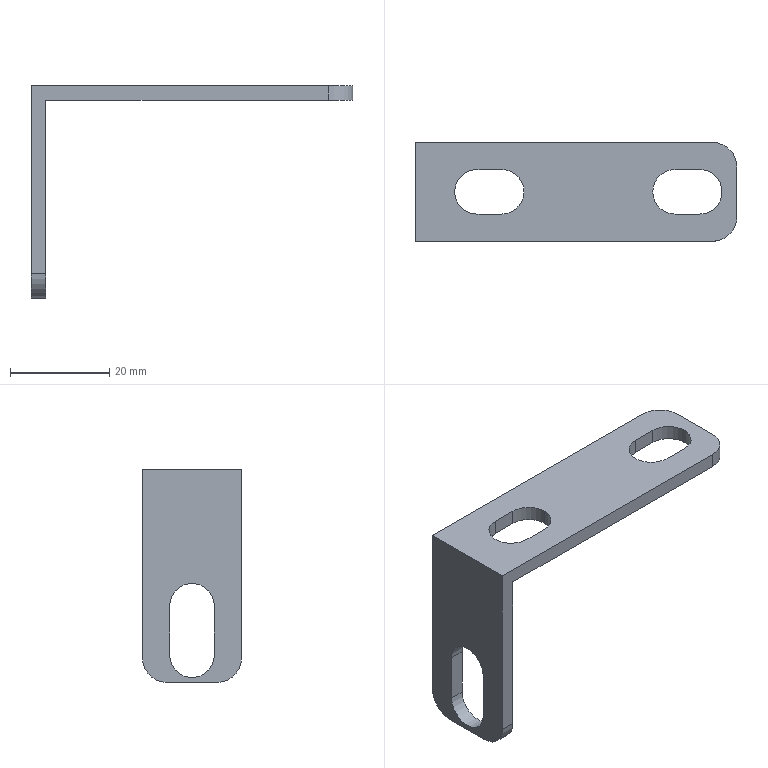Part | SolidWorks | features BaseBody 1 | 1 solid | 26 faces | box 65 x 20 x 43 mm | volume 5123 mm3 | plane 14 | cylinder 12 | commonest cylinder face diameters 9 x8 10 x4
STEP:
#1=CARTESIAN_POINT('',(15.5,0.,3.));
#2=VERTEX_POINT('',#1);
#3=CARTESIAN_POINT('',(20.,4.5,3.));
#4=VERTEX_POINT('',#3);
#5=CARTESIAN_POINT('',(20.,0.,3.));
#6=DIRECTION('',(0.,0.,-1.));
#7=DIRECTION('',(-1.,0.,0.));
#8=AXIS2_PLACEMENT_3D('',#5,#6,#7);
#9=CIRCLE('',#8,4.5);
#10=EDGE_CURVE('',#2,#4,#9,.T.);
#11=ORIENTED_EDGE('',*,*,#10,.F.);
#12=CARTESIAN_POINT('',(15.5,0.,0.));
#13=VERTEX_POINT('',#12);
#14=CARTESIAN_POINT('',(15.5,0.,3.));
#15=DIRECTION('',(0.,0.,-1.));
#16=VECTOR('',#15,1000.);
#17=LINE('',#14,#16);
#18=EDGE_CURVE('',#2,#13,#17,.T.);
#19=ORIENTED_EDGE('',*,*,#18,.T.);
#20=CARTESIAN_POINT('',(20.,4.5,0.));
#21=VERTEX_POINT('',#20);
#22=CARTESIAN_POINT('',(20.,0.,0.));
#23=DIRECTION('',(0.,0.,1.));
#24=DIRECTION('',(-1.,0.,0.));
#25=AXIS2_PLACEMENT_3D('',#22,#23,#24);
#26=CIRCLE('',#25,4.5);
#27=EDGE_CURVE('',#21,#13,#26,.T.);
#28=ORIENTED_EDGE('',*,*,#27,.F.);
#29=CARTESIAN_POINT('',(20.,4.5,3.));
#30=DIRECTION('',(0.,0.,1.));
#31=VECTOR('',#30,1000.);
#32=LINE('',#29,#31);
#33=EDGE_CURVE('',#21,#4,#32,.T.);
#34=ORIENTED_EDGE('',*,*,#33,.T.);
#35=EDGE_LOOP('',(#11,#19,#28,#34));
#36=FACE_OUTER_BOUND('',#35,.T.);
#37=CARTESIAN_POINT('',(20.,0.,3.));
#38=DIRECTION('',(0.,0.,-1.));
#39=DIRECTION('',(-1.,0.,0.));
#40=AXIS2_PLACEMENT_3D('',#37,#38,#39);
#41=CYLINDRICAL_SURFACE('',#40,4.5);
#42=ADVANCED_FACE('',(#36),#41,.F.);
#43=CARTESIAN_POINT('',(-10.5,0.,0.));
#44=VERTEX_POINT('',#43);
#45=CARTESIAN_POINT('',(-15.,4.5,0.));
#46=VERTEX_POINT('',#45);
#47=CARTESIAN_POINT('',(-15.,0.,0.));
#48=DIRECTION('',(0.,0.,1.));
#49=DIRECTION('',(1.,0.,0.));
#50=AXIS2_PLACEMENT_3D('',#47,#48,#49);
#51=CIRCLE('',#50,4.5);
#52=EDGE_CURVE('',#44,#46,#51,.T.);
#53=ORIENTED_EDGE('',*,*,#52,.F.);
#54=CARTESIAN_POINT('',(-10.5,0.,3.));
#55=VERTEX_POINT('',#54);
#56=CARTESIAN_POINT('',(-10.5,0.,-40.));
#57=DIRECTION('',(0.,0.,1.));
#58=VECTOR('',#57,1000.);
#59=LINE('',#56,#58);
#60=EDGE_CURVE('',#44,#55,#59,.T.);
#61=ORIENTED_EDGE('',*,*,#60,.T.);
#62=CARTESIAN_POINT('',(-15.,4.5,3.));
#63=VERTEX_POINT('',#62);
#64=CARTESIAN_POINT('',(-15.,0.,3.));
#65=DIRECTION('',(0.,0.,-1.));
#66=DIRECTION('',(1.,0.,0.));
#67=AXIS2_PLACEMENT_3D('',#64,#65,#66);
#68=CIRCLE('',#67,4.5);
#69=EDGE_CURVE('',#63,#55,#68,.T.);
#70=ORIENTED_EDGE('',*,*,#69,.F.);
#71=CARTESIAN_POINT('',(-15.,4.5,-40.));
#72=DIRECTION('',(0.,0.,1.));
#73=VECTOR('',#72,1000.);
#74=LINE('',#71,#73);
#75=EDGE_CURVE('',#46,#63,#74,.T.);
#76=ORIENTED_EDGE('',*,*,#75,.F.);
#77=EDGE_LOOP('',(#53,#61,#70,#76));
#78=FACE_OUTER_BOUND('',#77,.T.);
#79=CARTESIAN_POINT('',(-15.,0.,-40.));
#80=DIRECTION('',(0.,0.,1.));
#81=DIRECTION('',(1.,0.,0.));
#82=AXIS2_PLACEMENT_3D('',#79,#80,#81);
#83=CYLINDRICAL_SURFACE('',#82,4.5);
#84=ADVANCED_FACE('',(#78),#83,.F.);
#85=CARTESIAN_POINT('',(20.,-4.5,3.));
#86=VERTEX_POINT('',#85);
#87=CARTESIAN_POINT('',(20.,0.,3.));
#88=DIRECTION('',(0.,0.,-1.));
#89=DIRECTION('',(-1.,0.,0.));
#90=AXIS2_PLACEMENT_3D('',#87,#88,#89);
#91=CIRCLE('',#90,4.5);
#92=EDGE_CURVE('',#86,#2,#91,.T.);
#93=ORIENTED_EDGE('',*,*,#92,.T.);
#94=ORIENTED_EDGE('',*,*,#10,.T.);
#95=CARTESIAN_POINT('',(25.,4.5,3.));
#96=VERTEX_POINT('',#95);
#97=CARTESIAN_POINT('',(0.,4.5,3.));
#98=DIRECTION('',(1.,0.,0.));
#99=VECTOR('',#98,1000.);
#100=LINE('',#97,#99);
#101=EDGE_CURVE('',#4,#96,#100,.T.);
#102=ORIENTED_EDGE('',*,*,#101,.T.);
#103=CARTESIAN_POINT('',(25.,-4.5,3.));
#104=VERTEX_POINT('',#103);
#105=CARTESIAN_POINT('',(25.,0.,3.));
#106=DIRECTION('',(0.,0.,-1.));
#107=DIRECTION('',(-1.,0.,0.));
#108=AXIS2_PLACEMENT_3D('',#105,#106,#107);
#109=CIRCLE('',#108,4.5);
#110=EDGE_CURVE('',#96,#104,#109,.T.);
#111=ORIENTED_EDGE('',*,*,#110,.T.);
#112=CARTESIAN_POINT('',(0.,-4.5,3.));
#113=DIRECTION('',(-1.,0.,0.));
#114=VECTOR('',#113,1000.);
#115=LINE('',#112,#114);
#116=EDGE_CURVE('',#104,#86,#115,.T.);
#117=ORIENTED_EDGE('',*,*,#116,.T.);
#118=EDGE_LOOP('',(#93,#94,#102,#111,#117));
#119=FACE_BOUND('',#118,.T.);
#120=CARTESIAN_POINT('',(27.5,10.,3.));
#121=VERTEX_POINT('',#120);
#122=CARTESIAN_POINT('',(-32.5,10.,3.));
#123=VERTEX_POINT('',#122);
#124=CARTESIAN_POINT('',(0.,10.,3.));
#125=DIRECTION('',(-1.,0.,0.));
#126=VECTOR('',#125,1000.);
#127=LINE('',#124,#126);
#128=EDGE_CURVE('',#121,#123,#127,.T.);
#129=ORIENTED_EDGE('',*,*,#128,.T.);
#130=CARTESIAN_POINT('',(-32.5,-10.,3.));
#131=VERTEX_POINT('',#130);
#132=CARTESIAN_POINT('',(-32.5,0.,3.));
#133=DIRECTION('',(0.,-1.,0.));
#134=VECTOR('',#133,1000.);
#135=LINE('',#132,#134);
#136=EDGE_CURVE('',#123,#131,#135,.T.);
#137=ORIENTED_EDGE('',*,*,#136,.T.);
#138=CARTESIAN_POINT('',(27.5,-10.,3.));
#139=VERTEX_POINT('',#138);
#140=CARTESIAN_POINT('',(0.,-10.,3.));
#141=DIRECTION('',(1.,0.,0.));
#142=VECTOR('',#141,1000.);
#143=LINE('',#140,#142);
#144=EDGE_CURVE('',#131,#139,#143,.T.);
#145=ORIENTED_EDGE('',*,*,#144,.T.);
#146=CARTESIAN_POINT('',(32.5,-5.,3.));
#147=VERTEX_POINT('',#146);
#148=CARTESIAN_POINT('',(27.5,-5.,3.));
#149=DIRECTION('',(0.,0.,1.));
#150=DIRECTION('',(-1.,0.,0.));
#151=AXIS2_PLACEMENT_3D('',#148,#149,#150);
#152=CIRCLE('',#151,5.);
#153=EDGE_CURVE('',#139,#147,#152,.T.);
#154=ORIENTED_EDGE('',*,*,#153,.T.);
#155=CARTESIAN_POINT('',(32.5,5.,3.));
#156=VERTEX_POINT('',#155);
#157=CARTESIAN_POINT('',(32.5,0.,3.));
#158=DIRECTION('',(0.,1.,0.));
#159=VECTOR('',#158,1000.);
#160=LINE('',#157,#159);
#161=EDGE_CURVE('',#147,#156,#160,.T.);
#162=ORIENTED_EDGE('',*,*,#161,.T.);
#163=CARTESIAN_POINT('',(27.5,5.,3.));
#164=DIRECTION('',(0.,0.,1.));
#165=DIRECTION('',(1.,0.,0.));
#166=AXIS2_PLACEMENT_3D('',#163,#164,#165);
#167=CIRCLE('',#166,5.);
#168=EDGE_CURVE('',#156,#121,#167,.T.);
#169=ORIENTED_EDGE('',*,*,#168,.T.);
#170=EDGE_LOOP('',(#129,#137,#145,#154,#162,#169));
#171=FACE_OUTER_BOUND('',#170,.T.);
#172=ORIENTED_EDGE('',*,*,#69,.T.);
#173=CARTESIAN_POINT('',(-15.,-4.5,3.));
#174=VERTEX_POINT('',#173);
#175=CARTESIAN_POINT('',(-15.,0.,3.));
#176=DIRECTION('',(0.,0.,-1.));
#177=DIRECTION('',(1.,0.,0.));
#178=AXIS2_PLACEMENT_3D('',#175,#176,#177);
#179=CIRCLE('',#178,4.5);
#180=EDGE_CURVE('',#55,#174,#179,.T.);
#181=ORIENTED_EDGE('',*,*,#180,.T.);
#182=CARTESIAN_POINT('',(-20.,-4.5,3.));
#183=VERTEX_POINT('',#182);
#184=CARTESIAN_POINT('',(0.,-4.5,3.));
#185=DIRECTION('',(-1.,0.,0.));
#186=VECTOR('',#185,1000.);
#187=LINE('',#184,#186);
#188=EDGE_CURVE('',#174,#183,#187,.T.);
#189=ORIENTED_EDGE('',*,*,#188,.T.);
#190=CARTESIAN_POINT('',(-20.,4.5,3.));
#191=VERTEX_POINT('',#190);
#192=CARTESIAN_POINT('',(-20.,0.,3.));
#193=DIRECTION('',(0.,0.,-1.));
#194=DIRECTION('',(1.,0.,0.));
#195=AXIS2_PLACEMENT_3D('',#192,#193,#194);
#196=CIRCLE('',#195,4.5);
#197=EDGE_CURVE('',#183,#191,#196,.T.);
#198=ORIENTED_EDGE('',*,*,#197,.T.);
#199=CARTESIAN_POINT('',(0.,4.5,3.));
#200=DIRECTION('',(1.,0.,0.));
#201=VECTOR('',#200,1000.);
#202=LINE('',#199,#201);
#203=EDGE_CURVE('',#191,#63,#202,.T.);
#204=ORIENTED_EDGE('',*,*,#203,.T.);
#205=EDGE_LOOP('',(#172,#181,#189,#198,#204));
#206=FACE_BOUND('',#205,.T.);
#207=CARTESIAN_POINT('',(0.,0.,3.));
#208=DIRECTION('',(0.,0.,1.));
#209=DIRECTION('',(1.,0.,0.));
#210=AXIS2_PLACEMENT_3D('',#207,#208,#209);
#211=PLANE('',#210);
#212=ADVANCED_FACE('',(#119,#171,#206),#211,.T.);
#213=ORIENTED_EDGE('',*,*,#101,.F.);
#214=ORIENTED_EDGE('',*,*,#33,.F.);
#215=CARTESIAN_POINT('',(25.,4.5,0.));
#216=VERTEX_POINT('',#215);
#217=CARTESIAN_POINT('',(20.,4.5,0.));
#218=DIRECTION('',(-1.,0.,0.));
#219=VECTOR('',#218,1000.);
#220=LINE('',#217,#219);
#221=EDGE_CURVE('',#216,#21,#220,.T.);
#222=ORIENTED_EDGE('',*,*,#221,.F.);
#223=CARTESIAN_POINT('',(25.,4.5,3.));
#224=DIRECTION('',(0.,0.,-1.));
#225=VECTOR('',#224,1000.);
#226=LINE('',#223,#225);
#227=EDGE_CURVE('',#96,#216,#226,.T.);
#228=ORIENTED_EDGE('',*,*,#227,.F.);
#229=EDGE_LOOP('',(#213,#214,#222,#228));
#230=FACE_OUTER_BOUND('',#229,.T.);
#231=CARTESIAN_POINT('',(20.,4.5,3.));
#232=DIRECTION('',(0.,1.,0.));
#233=DIRECTION('',(-1.,0.,0.));
#234=AXIS2_PLACEMENT_3D('',#231,#232,#233);
#235=PLANE('',#234);
#236=ADVANCED_FACE('',(#230),#235,.F.);
#237=ORIENTED_EDGE('',*,*,#18,.F.);
#238=ORIENTED_EDGE('',*,*,#92,.F.);
#239=CARTESIAN_POINT('',(20.,-4.5,0.));
#240=VERTEX_POINT('',#239);
#241=CARTESIAN_POINT('',(20.,-4.5,3.));
#242=DIRECTION('',(0.,0.,1.));
#243=VECTOR('',#242,1000.);
#244=LINE('',#241,#243);
#245=EDGE_CURVE('',#240,#86,#244,.T.);
#246=ORIENTED_EDGE('',*,*,#245,.F.);
#247=CARTESIAN_POINT('',(20.,0.,0.));
#248=DIRECTION('',(0.,0.,1.));
#249=DIRECTION('',(-1.,0.,0.));
#250=AXIS2_PLACEMENT_3D('',#247,#248,#249);
#251=CIRCLE('',#250,4.5);
#252=EDGE_CURVE('',#13,#240,#251,.T.);
#253=ORIENTED_EDGE('',*,*,#252,.F.);
#254=EDGE_LOOP('',(#237,#238,#246,#253));
#255=FACE_OUTER_BOUND('',#254,.T.);
#256=CARTESIAN_POINT('',(20.,0.,3.));
#257=DIRECTION('',(0.,0.,-1.));
#258=DIRECTION('',(-1.,0.,0.));
#259=AXIS2_PLACEMENT_3D('',#256,#257,#258);
#260=CYLINDRICAL_SURFACE('',#259,4.5);
#261=ADVANCED_FACE('',(#255),#260,.F.);
#262=ORIENTED_EDGE('',*,*,#116,.F.);
#263=CARTESIAN_POINT('',(25.,-4.5,0.));
#264=VERTEX_POINT('',#263);
#265=CARTESIAN_POINT('',(25.,-4.5,3.));
#266=DIRECTION('',(0.,0.,1.));
#267=VECTOR('',#266,1000.);
#268=LINE('',#265,#267);
#269=EDGE_CURVE('',#264,#104,#268,.T.);
#270=ORIENTED_EDGE('',*,*,#269,.F.);
#271=CARTESIAN_POINT('',(20.,-4.5,0.));
#272=DIRECTION('',(1.,0.,0.));
#273=VECTOR('',#272,1000.);
#274=LINE('',#271,#273);
#275=EDGE_CURVE('',#240,#264,#274,.T.);
#276=ORIENTED_EDGE('',*,*,#275,.F.);
#277=ORIENTED_EDGE('',*,*,#245,.T.);
#278=EDGE_LOOP('',(#262,#270,#276,#277));
#279=FACE_OUTER_BOUND('',#278,.T.);
#280=CARTESIAN_POINT('',(20.,-4.5,3.));
#281=DIRECTION('',(0.,-1.,0.));
#282=DIRECTION('',(1.,0.,0.));
#283=AXIS2_PLACEMENT_3D('',#280,#281,#282);
#284=PLANE('',#283);
#285=ADVANCED_FACE('',(#279),#284,.F.);
#286=ORIENTED_EDGE('',*,*,#110,.F.);
#287=ORIENTED_EDGE('',*,*,#227,.T.);
#288=CARTESIAN_POINT('',(25.,0.,0.));
#289=DIRECTION('',(0.,0.,1.));
#290=DIRECTION('',(-1.,0.,0.));
#291=AXIS2_PLACEMENT_3D('',#288,#289,#290);
#292=CIRCLE('',#291,4.5);
#293=EDGE_CURVE('',#264,#216,#292,.T.);
#294=ORIENTED_EDGE('',*,*,#293,.F.);
#295=ORIENTED_EDGE('',*,*,#269,.T.);
#296=EDGE_LOOP('',(#286,#287,#294,#295));
#297=FACE_OUTER_BOUND('',#296,.T.);
#298=CARTESIAN_POINT('',(25.,0.,3.));
#299=DIRECTION('',(0.,0.,-1.));
#300=DIRECTION('',(-1.,0.,0.));
#301=AXIS2_PLACEMENT_3D('',#298,#299,#300);
#302=CYLINDRICAL_SURFACE('',#301,4.5);
#303=ADVANCED_FACE('',(#297),#302,.F.);
#304=CARTESIAN_POINT('',(-32.5,-4.5,-34.5));
#305=VERTEX_POINT('',#304);
#306=CARTESIAN_POINT('',(-32.5,-4.5,-24.5));
#307=VERTEX_POINT('',#306);
#308=CARTESIAN_POINT('',(-32.5,-4.5,3.));
#309=DIRECTION('',(0.,0.,1.));
#310=VECTOR('',#309,1000.);
#311=LINE('',#308,#310);
#312=EDGE_CURVE('',#305,#307,#311,.T.);
#313=ORIENTED_EDGE('',*,*,#312,.F.);
#314=CARTESIAN_POINT('',(-32.5,4.5,-34.5));
#315=VERTEX_POINT('',#314);
#316=CARTESIAN_POINT('',(-32.5,0.,-34.5));
#317=DIRECTION('',(-1.,0.,0.));
#318=DIRECTION('',(0.,1.,0.));
#319=AXIS2_PLACEMENT_3D('',#316,#317,#318);
#320=CIRCLE('',#319,4.5);
#321=EDGE_CURVE('',#315,#305,#320,.T.);
#322=ORIENTED_EDGE('',*,*,#321,.F.);
#323=CARTESIAN_POINT('',(-32.5,4.5,-24.5));
#324=VERTEX_POINT('',#323);
#325=CARTESIAN_POINT('',(-32.5,4.5,3.));
#326=DIRECTION('',(0.,0.,-1.));
#327=VECTOR('',#326,1000.);
#328=LINE('',#325,#327);
#329=EDGE_CURVE('',#324,#315,#328,.T.);
#330=ORIENTED_EDGE('',*,*,#329,.F.);
#331=CARTESIAN_POINT('',(-32.5,0.,-24.5));
#332=DIRECTION('',(-1.,0.,0.));
#333=DIRECTION('',(0.,1.,0.));
#334=AXIS2_PLACEMENT_3D('',#331,#332,#333);
#335=CIRCLE('',#334,4.5);
#336=EDGE_CURVE('',#307,#324,#335,.T.);
#337=ORIENTED_EDGE('',*,*,#336,.F.);
#338=EDGE_LOOP('',(#313,#322,#330,#337));
#339=FACE_BOUND('',#338,.T.);
#340=CARTESIAN_POINT('',(-32.5,5.,-40.));
#341=VERTEX_POINT('',#340);
#342=CARTESIAN_POINT('',(-32.5,10.,-35.));
#343=VERTEX_POINT('',#342);
#344=CARTESIAN_POINT('',(-32.5,5.,-35.));
#345=DIRECTION('',(1.,0.,0.));
#346=DIRECTION('',(0.,0.,-1.));
#347=AXIS2_PLACEMENT_3D('',#344,#345,#346);
#348=CIRCLE('',#347,5.);
#349=EDGE_CURVE('',#341,#343,#348,.T.);
#350=ORIENTED_EDGE('',*,*,#349,.F.);
#351=CARTESIAN_POINT('',(-32.5,-5.,-40.));
#352=VERTEX_POINT('',#351);
#353=CARTESIAN_POINT('',(-32.5,10.,-40.));
#354=DIRECTION('',(0.,1.,0.));
#355=VECTOR('',#354,1000.);
#356=LINE('',#353,#355);
#357=EDGE_CURVE('',#352,#341,#356,.T.);
#358=ORIENTED_EDGE('',*,*,#357,.F.);
#359=CARTESIAN_POINT('',(-32.5,-10.,-35.));
#360=VERTEX_POINT('',#359);
#361=CARTESIAN_POINT('',(-32.5,-5.,-35.));
#362=DIRECTION('',(1.,0.,0.));
#363=DIRECTION('',(0.,0.,1.));
#364=AXIS2_PLACEMENT_3D('',#361,#362,#363);
#365=CIRCLE('',#364,5.);
#366=EDGE_CURVE('',#360,#352,#365,.T.);
#367=ORIENTED_EDGE('',*,*,#366,.F.);
#368=CARTESIAN_POINT('',(-32.5,-10.,3.));
#369=DIRECTION('',(0.,0.,-1.));
#370=VECTOR('',#369,1000.);
#371=LINE('',#368,#370);
#372=EDGE_CURVE('',#131,#360,#371,.T.);
#373=ORIENTED_EDGE('',*,*,#372,.F.);
#374=ORIENTED_EDGE('',*,*,#136,.F.);
#375=CARTESIAN_POINT('',(-32.5,10.,3.));
#376=DIRECTION('',(0.,0.,1.));
#377=VECTOR('',#376,1000.);
#378=LINE('',#375,#377);
#379=EDGE_CURVE('',#343,#123,#378,.T.);
#380=ORIENTED_EDGE('',*,*,#379,.F.);
#381=EDGE_LOOP('',(#350,#358,#367,#373,#374,#380));
#382=FACE_OUTER_BOUND('',#381,.T.);
#383=CARTESIAN_POINT('',(-32.5,10.,3.));
#384=DIRECTION('',(1.,0.,0.));
#385=DIRECTION('',(0.,0.,-1.));
#386=AXIS2_PLACEMENT_3D('',#383,#384,#385);
#387=PLANE('',#386);
#388=ADVANCED_FACE('',(#339,#382),#387,.F.);
#389=CARTESIAN_POINT('',(-29.5,10.,-35.));
#390=VERTEX_POINT('',#389);
#391=CARTESIAN_POINT('',(-32.5,10.,-35.));
#392=DIRECTION('',(1.,0.,0.));
#393=VECTOR('',#392,1000.);
#394=LINE('',#391,#393);
#395=EDGE_CURVE('',#343,#390,#394,.T.);
#396=ORIENTED_EDGE('',*,*,#395,.F.);
#397=ORIENTED_EDGE('',*,*,#379,.T.);
#398=ORIENTED_EDGE('',*,*,#128,.F.);
#399=CARTESIAN_POINT('',(27.5,10.,0.));
#400=VERTEX_POINT('',#399);
#401=CARTESIAN_POINT('',(27.5,10.,3.));
#402=DIRECTION('',(0.,0.,1.));
#403=VECTOR('',#402,1000.);
#404=LINE('',#401,#403);
#405=EDGE_CURVE('',#400,#121,#404,.T.);
#406=ORIENTED_EDGE('',*,*,#405,.F.);
#407=CARTESIAN_POINT('',(-29.5,10.,0.));
#408=VERTEX_POINT('',#407);
#409=CARTESIAN_POINT('',(-32.5,10.,0.));
#410=DIRECTION('',(1.,0.,0.));
#411=VECTOR('',#410,1000.);
#412=LINE('',#409,#411);
#413=EDGE_CURVE('',#408,#400,#412,.T.);
#414=ORIENTED_EDGE('',*,*,#413,.F.);
#415=CARTESIAN_POINT('',(-29.5,10.,3.));
#416=DIRECTION('',(0.,0.,1.));
#417=VECTOR('',#416,1000.);
#418=LINE('',#415,#417);
#419=EDGE_CURVE('',#390,#408,#418,.T.);
#420=ORIENTED_EDGE('',*,*,#419,.F.);
#421=EDGE_LOOP('',(#396,#397,#398,#406,#414,#420));
#422=FACE_OUTER_BOUND('',#421,.T.);
#423=CARTESIAN_POINT('',(-32.5,10.,3.));
#424=DIRECTION('',(0.,-1.,0.));
#425=DIRECTION('',(0.,0.,-1.));
#426=AXIS2_PLACEMENT_3D('',#423,#424,#425);
#427=PLANE('',#426);
#428=ADVANCED_FACE('',(#422),#427,.F.);
#429=ORIENTED_EDGE('',*,*,#168,.F.);
#430=CARTESIAN_POINT('',(32.5,5.,0.));
#431=VERTEX_POINT('',#430);
#432=CARTESIAN_POINT('',(32.5,5.,3.));
#433=DIRECTION('',(0.,0.,-1.));
#434=VECTOR('',#433,1000.);
#435=LINE('',#432,#434);
#436=EDGE_CURVE('',#156,#431,#435,.T.);
#437=ORIENTED_EDGE('',*,*,#436,.T.);
#438=CARTESIAN_POINT('',(27.5,5.,0.));
#439=DIRECTION('',(0.,0.,1.));
#440=DIRECTION('',(1.,0.,0.));
#441=AXIS2_PLACEMENT_3D('',#438,#439,#440);
#442=CIRCLE('',#441,5.);
#443=EDGE_CURVE('',#431,#400,#442,.T.);
#444=ORIENTED_EDGE('',*,*,#443,.T.);
#445=ORIENTED_EDGE('',*,*,#405,.T.);
#446=EDGE_LOOP('',(#429,#437,#444,#445));
#447=FACE_OUTER_BOUND('',#446,.T.);
#448=CARTESIAN_POINT('',(27.5,5.,3.));
#449=DIRECTION('',(0.,0.,1.));
#450=DIRECTION('',(1.,0.,0.));
#451=AXIS2_PLACEMENT_3D('',#448,#449,#450);
#452=CYLINDRICAL_SURFACE('',#451,5.);
#453=ADVANCED_FACE('',(#447),#452,.T.);
#454=CARTESIAN_POINT('',(32.5,-5.,0.));
#455=VERTEX_POINT('',#454);
#456=CARTESIAN_POINT('',(32.5,-5.,3.));
#457=DIRECTION('',(0.,0.,1.));
#458=VECTOR('',#457,1000.);
#459=LINE('',#456,#458);
#460=EDGE_CURVE('',#455,#147,#459,.T.);
#461=ORIENTED_EDGE('',*,*,#460,.F.);
#462=CARTESIAN_POINT('',(32.5,10.,0.));
#463=DIRECTION('',(0.,-1.,0.));
#464=VECTOR('',#463,1000.);
#465=LINE('',#462,#464);
#466=EDGE_CURVE('',#431,#455,#465,.T.);
#467=ORIENTED_EDGE('',*,*,#466,.F.);
#468=ORIENTED_EDGE('',*,*,#436,.F.);
#469=ORIENTED_EDGE('',*,*,#161,.F.);
#470=EDGE_LOOP('',(#461,#467,#468,#469));
#471=FACE_OUTER_BOUND('',#470,.T.);
#472=CARTESIAN_POINT('',(32.5,10.,3.));
#473=DIRECTION('',(-1.,0.,0.));
#474=DIRECTION('',(0.,0.,1.));
#475=AXIS2_PLACEMENT_3D('',#472,#473,#474);
#476=PLANE('',#475);
#477=ADVANCED_FACE('',(#471),#476,.F.);
#478=CARTESIAN_POINT('',(27.5,-10.,0.));
#479=VERTEX_POINT('',#478);
#480=CARTESIAN_POINT('',(27.5,-5.,0.));
#481=DIRECTION('',(0.,0.,1.));
#482=DIRECTION('',(-1.,0.,0.));
#483=AXIS2_PLACEMENT_3D('',#480,#481,#482);
#484=CIRCLE('',#483,5.);
#485=EDGE_CURVE('',#479,#455,#484,.T.);
#486=ORIENTED_EDGE('',*,*,#485,.T.);
#487=ORIENTED_EDGE('',*,*,#460,.T.);
#488=ORIENTED_EDGE('',*,*,#153,.F.);
#489=CARTESIAN_POINT('',(27.5,-10.,3.));
#490=DIRECTION('',(0.,0.,-1.));
#491=VECTOR('',#490,1000.);
#492=LINE('',#489,#491);
#493=EDGE_CURVE('',#139,#479,#492,.T.);
#494=ORIENTED_EDGE('',*,*,#493,.T.);
#495=EDGE_LOOP('',(#486,#487,#488,#494));
#496=FACE_OUTER_BOUND('',#495,.T.);
#497=CARTESIAN_POINT('',(27.5,-5.,3.));
#498=DIRECTION('',(0.,0.,-1.));
#499=DIRECTION('',(-1.,0.,0.));
#500=AXIS2_PLACEMENT_3D('',#497,#498,#499);
#501=CYLINDRICAL_SURFACE('',#500,5.);
#502=ADVANCED_FACE('',(#496),#501,.T.);
#503=CARTESIAN_POINT('',(-29.5,-10.,-35.));
#504=VERTEX_POINT('',#503);
#505=CARTESIAN_POINT('',(-32.5,-10.,-35.));
#506=DIRECTION('',(-1.,0.,0.));
#507=VECTOR('',#506,1000.);
#508=LINE('',#505,#507);
#509=EDGE_CURVE('',#504,#360,#508,.T.);
#510=ORIENTED_EDGE('',*,*,#509,.F.);
#511=CARTESIAN_POINT('',(-29.5,-10.,0.));
#512=VERTEX_POINT('',#511);
#513=CARTESIAN_POINT('',(-29.5,-10.,3.));
#514=DIRECTION('',(0.,0.,-1.));
#515=VECTOR('',#514,1000.);
#516=LINE('',#513,#515);
#517=EDGE_CURVE('',#512,#504,#516,.T.);
#518=ORIENTED_EDGE('',*,*,#517,.F.);
#519=CARTESIAN_POINT('',(-32.5,-10.,0.));
#520=DIRECTION('',(-1.,0.,0.));
#521=VECTOR('',#520,1000.);
#522=LINE('',#519,#521);
#523=EDGE_CURVE('',#479,#512,#522,.T.);
#524=ORIENTED_EDGE('',*,*,#523,.F.);
#525=ORIENTED_EDGE('',*,*,#493,.F.);
#526=ORIENTED_EDGE('',*,*,#144,.F.);
#527=ORIENTED_EDGE('',*,*,#372,.T.);
#528=EDGE_LOOP('',(#510,#518,#524,#525,#526,#527));
#529=FACE_OUTER_BOUND('',#528,.T.);
#530=CARTESIAN_POINT('',(-32.5,-10.,3.));
#531=DIRECTION('',(0.,1.,0.));
#532=DIRECTION('',(0.,0.,1.));
#533=AXIS2_PLACEMENT_3D('',#530,#531,#532);
#534=PLANE('',#533);
#535=ADVANCED_FACE('',(#529),#534,.F.);
#536=ORIENTED_EDGE('',*,*,#188,.F.);
#537=CARTESIAN_POINT('',(-15.,-4.5,0.));
#538=VERTEX_POINT('',#537);
#539=CARTESIAN_POINT('',(-15.,-4.5,-40.));
#540=DIRECTION('',(0.,0.,1.));
#541=VECTOR('',#540,1000.);
#542=LINE('',#539,#541);
#543=EDGE_CURVE('',#538,#174,#542,.T.);
#544=ORIENTED_EDGE('',*,*,#543,.F.);
#545=CARTESIAN_POINT('',(-20.,-4.5,0.));
#546=VERTEX_POINT('',#545);
#547=CARTESIAN_POINT('',(-20.,-4.5,0.));
#548=DIRECTION('',(1.,0.,0.));
#549=VECTOR('',#548,1000.);
#550=LINE('',#547,#549);
#551=EDGE_CURVE('',#546,#538,#550,.T.);
#552=ORIENTED_EDGE('',*,*,#551,.F.);
#553=CARTESIAN_POINT('',(-20.,-4.5,-40.));
#554=DIRECTION('',(0.,0.,-1.));
#555=VECTOR('',#554,1000.);
#556=LINE('',#553,#555);
#557=EDGE_CURVE('',#183,#546,#556,.T.);
#558=ORIENTED_EDGE('',*,*,#557,.F.);
#559=EDGE_LOOP('',(#536,#544,#552,#558));
#560=FACE_OUTER_BOUND('',#559,.T.);
#561=CARTESIAN_POINT('',(-20.,-4.5,-40.));
#562=DIRECTION('',(0.,-1.,0.));
#563=DIRECTION('',(0.,0.,-1.));
#564=AXIS2_PLACEMENT_3D('',#561,#562,#563);
#565=PLANE('',#564);
#566=ADVANCED_FACE('',(#560),#565,.F.);
#567=ORIENTED_EDGE('',*,*,#60,.F.);
#568=CARTESIAN_POINT('',(-15.,0.,0.));
#569=DIRECTION('',(0.,0.,1.));
#570=DIRECTION('',(1.,0.,0.));
#571=AXIS2_PLACEMENT_3D('',#568,#569,#570);
#572=CIRCLE('',#571,4.5);
#573=EDGE_CURVE('',#538,#44,#572,.T.);
#574=ORIENTED_EDGE('',*,*,#573,.F.);
#575=ORIENTED_EDGE('',*,*,#543,.T.);
#576=ORIENTED_EDGE('',*,*,#180,.F.);
#577=EDGE_LOOP('',(#567,#574,#575,#576));
#578=FACE_OUTER_BOUND('',#577,.T.);
#579=CARTESIAN_POINT('',(-15.,0.,-40.));
#580=DIRECTION('',(0.,0.,1.));
#581=DIRECTION('',(1.,0.,0.));
#582=AXIS2_PLACEMENT_3D('',#579,#580,#581);
#583=CYLINDRICAL_SURFACE('',#582,4.5);
#584=ADVANCED_FACE('',(#578),#583,.F.);
#585=ORIENTED_EDGE('',*,*,#203,.F.);
#586=CARTESIAN_POINT('',(-20.,4.5,0.));
#587=VERTEX_POINT('',#586);
#588=CARTESIAN_POINT('',(-20.,4.5,-40.));
#589=DIRECTION('',(0.,0.,1.));
#590=VECTOR('',#589,1000.);
#591=LINE('',#588,#590);
#592=EDGE_CURVE('',#587,#191,#591,.T.);
#593=ORIENTED_EDGE('',*,*,#592,.F.);
#594=CARTESIAN_POINT('',(-20.,4.5,0.));
#595=DIRECTION('',(-1.,0.,0.));
#596=VECTOR('',#595,1000.);
#597=LINE('',#594,#596);
#598=EDGE_CURVE('',#46,#587,#597,.T.);
#599=ORIENTED_EDGE('',*,*,#598,.F.);
#600=ORIENTED_EDGE('',*,*,#75,.T.);
#601=EDGE_LOOP('',(#585,#593,#599,#600));
#602=FACE_OUTER_BOUND('',#601,.T.);
#603=CARTESIAN_POINT('',(-20.,4.5,-40.));
#604=DIRECTION('',(0.,1.,0.));
#605=DIRECTION('',(0.,0.,1.));
#606=AXIS2_PLACEMENT_3D('',#603,#604,#605);
#607=PLANE('',#606);
#608=ADVANCED_FACE('',(#602),#607,.F.);
#609=ORIENTED_EDGE('',*,*,#197,.F.);
#610=ORIENTED_EDGE('',*,*,#557,.T.);
#611=CARTESIAN_POINT('',(-20.,0.,0.));
#612=DIRECTION('',(0.,0.,1.));
#613=DIRECTION('',(1.,0.,0.));
#614=AXIS2_PLACEMENT_3D('',#611,#612,#613);
#615=CIRCLE('',#614,4.5);
#616=EDGE_CURVE('',#587,#546,#615,.T.);
#617=ORIENTED_EDGE('',*,*,#616,.F.);
#618=ORIENTED_EDGE('',*,*,#592,.T.);
#619=EDGE_LOOP('',(#609,#610,#617,#618));
#620=FACE_OUTER_BOUND('',#619,.T.);
#621=CARTESIAN_POINT('',(-20.,0.,-40.));
#622=DIRECTION('',(0.,0.,1.));
#623=DIRECTION('',(1.,0.,0.));
#624=AXIS2_PLACEMENT_3D('',#621,#622,#623);
#625=CYLINDRICAL_SURFACE('',#624,4.5);
#626=ADVANCED_FACE('',(#620),#625,.F.);
#627=ORIENTED_EDGE('',*,*,#27,.T.);
#628=ORIENTED_EDGE('',*,*,#252,.T.);
#629=ORIENTED_EDGE('',*,*,#275,.T.);
#630=ORIENTED_EDGE('',*,*,#293,.T.);
#631=ORIENTED_EDGE('',*,*,#221,.T.);
#632=EDGE_LOOP('',(#627,#628,#629,#630,#631));
#633=FACE_BOUND('',#632,.T.);
#634=ORIENTED_EDGE('',*,*,#485,.F.);
#635=ORIENTED_EDGE('',*,*,#523,.T.);
#636=CARTESIAN_POINT('',(-29.5,0.,0.));
#637=DIRECTION('',(0.,-1.,0.));
#638=VECTOR('',#637,1000.);
#639=LINE('',#636,#638);
#640=EDGE_CURVE('',#408,#512,#639,.T.);
#641=ORIENTED_EDGE('',*,*,#640,.F.);
#642=ORIENTED_EDGE('',*,*,#413,.T.);
#643=ORIENTED_EDGE('',*,*,#443,.F.);
#644=ORIENTED_EDGE('',*,*,#466,.T.);
#645=EDGE_LOOP('',(#634,#635,#641,#642,#643,#644));
#646=FACE_OUTER_BOUND('',#645,.T.);
#647=ORIENTED_EDGE('',*,*,#616,.T.);
#648=ORIENTED_EDGE('',*,*,#551,.T.);
#649=ORIENTED_EDGE('',*,*,#573,.T.);
#650=ORIENTED_EDGE('',*,*,#52,.T.);
#651=ORIENTED_EDGE('',*,*,#598,.T.);
#652=EDGE_LOOP('',(#647,#648,#649,#650,#651));
#653=FACE_BOUND('',#652,.T.);
#654=CARTESIAN_POINT('',(0.,0.,0.));
#655=DIRECTION('',(0.,0.,1.));
#656=DIRECTION('',(1.,0.,0.));
#657=AXIS2_PLACEMENT_3D('',#654,#655,#656);
#658=PLANE('',#657);
#659=ADVANCED_FACE('',(#633,#646,#653),#658,.F.);
#660=ORIENTED_EDGE('',*,*,#336,.T.);
#661=CARTESIAN_POINT('',(-29.5,4.5,-24.5));
#662=VERTEX_POINT('',#661);
#663=CARTESIAN_POINT('',(-32.5,4.5,-24.5));
#664=DIRECTION('',(-1.,0.,0.));
#665=VECTOR('',#664,1000.);
#666=LINE('',#663,#665);
#667=EDGE_CURVE('',#662,#324,#666,.T.);
#668=ORIENTED_EDGE('',*,*,#667,.F.);
#669=CARTESIAN_POINT('',(-29.5,-4.5,-24.5));
#670=VERTEX_POINT('',#669);
#671=CARTESIAN_POINT('',(-29.5,0.,-24.5));
#672=DIRECTION('',(-1.,0.,0.));
#673=DIRECTION('',(0.,1.,0.));
#674=AXIS2_PLACEMENT_3D('',#671,#672,#673);
#675=CIRCLE('',#674,4.5);
#676=EDGE_CURVE('',#670,#662,#675,.T.);
#677=ORIENTED_EDGE('',*,*,#676,.F.);
#678=CARTESIAN_POINT('',(-32.5,-4.5,-24.5));
#679=DIRECTION('',(1.,0.,0.));
#680=VECTOR('',#679,1000.);
#681=LINE('',#678,#680);
#682=EDGE_CURVE('',#307,#670,#681,.T.);
#683=ORIENTED_EDGE('',*,*,#682,.F.);
#684=EDGE_LOOP('',(#660,#668,#677,#683));
#685=FACE_OUTER_BOUND('',#684,.T.);
#686=CARTESIAN_POINT('',(-32.5,0.,-24.5));
#687=DIRECTION('',(1.,0.,0.));
#688=DIRECTION('',(0.,1.,0.));
#689=AXIS2_PLACEMENT_3D('',#686,#687,#688);
#690=CYLINDRICAL_SURFACE('',#689,4.5);
#691=ADVANCED_FACE('',(#685),#690,.F.);
#692=ORIENTED_EDGE('',*,*,#312,.T.);
#693=ORIENTED_EDGE('',*,*,#682,.T.);
#694=CARTESIAN_POINT('',(-29.5,-4.5,-34.5));
#695=VERTEX_POINT('',#694);
#696=CARTESIAN_POINT('',(-29.5,-4.5,-29.5));
#697=DIRECTION('',(0.,0.,1.));
#698=VECTOR('',#697,1000.);
#699=LINE('',#696,#698);
#700=EDGE_CURVE('',#695,#670,#699,.T.);
#701=ORIENTED_EDGE('',*,*,#700,.F.);
#702=CARTESIAN_POINT('',(-32.5,-4.5,-34.5));
#703=DIRECTION('',(1.,0.,0.));
#704=VECTOR('',#703,1000.);
#705=LINE('',#702,#704);
#706=EDGE_CURVE('',#305,#695,#705,.T.);
#707=ORIENTED_EDGE('',*,*,#706,.F.);
#708=EDGE_LOOP('',(#692,#693,#701,#707));
#709=FACE_OUTER_BOUND('',#708,.T.);
#710=CARTESIAN_POINT('',(-32.5,-4.5,-29.5));
#711=DIRECTION('',(0.,-1.,0.));
#712=DIRECTION('',(0.,0.,-1.));
#713=AXIS2_PLACEMENT_3D('',#710,#711,#712);
#714=PLANE('',#713);
#715=ADVANCED_FACE('',(#709),#714,.F.);
#716=ORIENTED_EDGE('',*,*,#321,.T.);
#717=ORIENTED_EDGE('',*,*,#706,.T.);
#718=CARTESIAN_POINT('',(-29.5,4.5,-34.5));
#719=VERTEX_POINT('',#718);
#720=CARTESIAN_POINT('',(-29.5,0.,-34.5));
#721=DIRECTION('',(-1.,0.,0.));
#722=DIRECTION('',(0.,1.,0.));
#723=AXIS2_PLACEMENT_3D('',#720,#721,#722);
#724=CIRCLE('',#723,4.5);
#725=EDGE_CURVE('',#719,#695,#724,.T.);
#726=ORIENTED_EDGE('',*,*,#725,.F.);
#727=CARTESIAN_POINT('',(-32.5,4.5,-34.5));
#728=DIRECTION('',(1.,0.,0.));
#729=VECTOR('',#728,1000.);
#730=LINE('',#727,#729);
#731=EDGE_CURVE('',#315,#719,#730,.T.);
#732=ORIENTED_EDGE('',*,*,#731,.F.);
#733=EDGE_LOOP('',(#716,#717,#726,#732));
#734=FACE_OUTER_BOUND('',#733,.T.);
#735=CARTESIAN_POINT('',(-32.5,0.,-34.5));
#736=DIRECTION('',(1.,0.,0.));
#737=DIRECTION('',(0.,1.,0.));
#738=AXIS2_PLACEMENT_3D('',#735,#736,#737);
#739=CYLINDRICAL_SURFACE('',#738,4.5);
#740=ADVANCED_FACE('',(#734),#739,.F.);
#741=ORIENTED_EDGE('',*,*,#329,.T.);
#742=ORIENTED_EDGE('',*,*,#731,.T.);
#743=CARTESIAN_POINT('',(-29.5,4.5,-29.5));
#744=DIRECTION('',(0.,0.,-1.));
#745=VECTOR('',#744,1000.);
#746=LINE('',#743,#745);
#747=EDGE_CURVE('',#662,#719,#746,.T.);
#748=ORIENTED_EDGE('',*,*,#747,.F.);
#749=ORIENTED_EDGE('',*,*,#667,.T.);
#750=EDGE_LOOP('',(#741,#742,#748,#749));
#751=FACE_OUTER_BOUND('',#750,.T.);
#752=CARTESIAN_POINT('',(-32.5,4.5,-29.5));
#753=DIRECTION('',(0.,1.,0.));
#754=DIRECTION('',(0.,0.,1.));
#755=AXIS2_PLACEMENT_3D('',#752,#753,#754);
#756=PLANE('',#755);
#757=ADVANCED_FACE('',(#751),#756,.F.);
#758=CARTESIAN_POINT('',(-29.5,5.,-40.));
#759=VERTEX_POINT('',#758);
#760=CARTESIAN_POINT('',(-29.5,5.,-35.));
#761=DIRECTION('',(-1.,0.,0.));
#762=DIRECTION('',(0.,0.,-1.));
#763=AXIS2_PLACEMENT_3D('',#760,#761,#762);
#764=CIRCLE('',#763,5.);
#765=EDGE_CURVE('',#390,#759,#764,.T.);
#766=ORIENTED_EDGE('',*,*,#765,.T.);
#767=CARTESIAN_POINT('',(0.,5.,-40.));
#768=DIRECTION('',(-1.,0.,0.));
#769=VECTOR('',#768,1000.);
#770=LINE('',#767,#769);
#771=EDGE_CURVE('',#759,#341,#770,.T.);
#772=ORIENTED_EDGE('',*,*,#771,.T.);
#773=ORIENTED_EDGE('',*,*,#349,.T.);
#774=ORIENTED_EDGE('',*,*,#395,.T.);
#775=EDGE_LOOP('',(#766,#772,#773,#774));
#776=FACE_OUTER_BOUND('',#775,.T.);
#777=CARTESIAN_POINT('',(0.,5.,-35.));
#778=DIRECTION('',(1.,0.,0.));
#779=DIRECTION('',(0.,0.,-1.));
#780=AXIS2_PLACEMENT_3D('',#777,#778,#779);
#781=CYLINDRICAL_SURFACE('',#780,5.);
#782=ADVANCED_FACE('',(#776),#781,.T.);
#783=ORIENTED_EDGE('',*,*,#771,.F.);
#784=CARTESIAN_POINT('',(-29.5,-5.,-40.));
#785=VERTEX_POINT('',#784);
#786=CARTESIAN_POINT('',(-29.5,0.,-40.));
#787=DIRECTION('',(0.,1.,0.));
#788=VECTOR('',#787,1000.);
#789=LINE('',#786,#788);
#790=EDGE_CURVE('',#785,#759,#789,.T.);
#791=ORIENTED_EDGE('',*,*,#790,.F.);
#792=CARTESIAN_POINT('',(0.,-5.,-40.));
#793=DIRECTION('',(1.,0.,0.));
#794=VECTOR('',#793,1000.);
#795=LINE('',#792,#794);
#796=EDGE_CURVE('',#352,#785,#795,.T.);
#797=ORIENTED_EDGE('',*,*,#796,.F.);
#798=ORIENTED_EDGE('',*,*,#357,.T.);
#799=EDGE_LOOP('',(#783,#791,#797,#798));
#800=FACE_OUTER_BOUND('',#799,.T.);
#801=CARTESIAN_POINT('',(0.,0.,-40.));
#802=DIRECTION('',(0.,0.,1.));
#803=DIRECTION('',(1.,0.,0.));
#804=AXIS2_PLACEMENT_3D('',#801,#802,#803);
#805=PLANE('',#804);
#806=ADVANCED_FACE('',(#800),#805,.F.);
#807=ORIENTED_EDGE('',*,*,#366,.T.);
#808=ORIENTED_EDGE('',*,*,#796,.T.);
#809=CARTESIAN_POINT('',(-29.5,-5.,-35.));
#810=DIRECTION('',(-1.,0.,0.));
#811=DIRECTION('',(0.,0.,1.));
#812=AXIS2_PLACEMENT_3D('',#809,#810,#811);
#813=CIRCLE('',#812,5.);
#814=EDGE_CURVE('',#785,#504,#813,.T.);
#815=ORIENTED_EDGE('',*,*,#814,.T.);
#816=ORIENTED_EDGE('',*,*,#509,.T.);
#817=EDGE_LOOP('',(#807,#808,#815,#816));
#818=FACE_OUTER_BOUND('',#817,.T.);
#819=CARTESIAN_POINT('',(0.,-5.,-35.));
#820=DIRECTION('',(-1.,0.,0.));
#821=DIRECTION('',(0.,0.,1.));
#822=AXIS2_PLACEMENT_3D('',#819,#820,#821);
#823=CYLINDRICAL_SURFACE('',#822,5.);
#824=ADVANCED_FACE('',(#818),#823,.T.);
#825=ORIENTED_EDGE('',*,*,#747,.T.);
#826=ORIENTED_EDGE('',*,*,#725,.T.);
#827=ORIENTED_EDGE('',*,*,#700,.T.);
#828=ORIENTED_EDGE('',*,*,#676,.T.);
#829=EDGE_LOOP('',(#825,#826,#827,#828));
#830=FACE_BOUND('',#829,.T.);
#831=ORIENTED_EDGE('',*,*,#765,.F.);
#832=ORIENTED_EDGE('',*,*,#419,.T.);
#833=ORIENTED_EDGE('',*,*,#640,.T.);
#834=ORIENTED_EDGE('',*,*,#517,.T.);
#835=ORIENTED_EDGE('',*,*,#814,.F.);
#836=ORIENTED_EDGE('',*,*,#790,.T.);
#837=EDGE_LOOP('',(#831,#832,#833,#834,#835,#836));
#838=FACE_OUTER_BOUND('',#837,.T.);
#839=CARTESIAN_POINT('',(-29.5,10.,-40.));
#840=DIRECTION('',(-1.,0.,0.));
#841=DIRECTION('',(0.,-1.,0.));
#842=AXIS2_PLACEMENT_3D('',#839,#840,#841);
#843=PLANE('',#842);
#844=ADVANCED_FACE('',(#830,#838),#843,.F.);
#845=CLOSED_SHELL('',(#42,#84,#212,#236,#261,#285,#303,#388,#428,#453,#477,#502,#535,#566,#584,#608,#626,#659,#691,#715,#740,#757,#782,#806,#824,#844));
#846=MANIFOLD_SOLID_BREP('',#845);
#847=CARTESIAN_POINT('',(0.,0.,0.));
#848=DIRECTION('',(0.,0.,1.));
#849=DIRECTION('',(1.,0.,0.));
#850=AXIS2_PLACEMENT_3D('',#847,#848,#849);
#851=(LENGTH_UNIT()NAMED_UNIT(*)SI_UNIT(.MILLI.,.METRE.));
#852=UNCERTAINTY_MEASURE_WITH_UNIT(LENGTH_MEASURE(0.00001),#851,'','');
#853=(NAMED_UNIT(*)PLANE_ANGLE_UNIT()SI_UNIT($,.RADIAN.));
#854=(NAMED_UNIT(*)SI_UNIT($,.STERADIAN.)SOLID_ANGLE_UNIT());
#855=(GEOMETRIC_REPRESENTATION_CONTEXT(3)GLOBAL_UNCERTAINTY_ASSIGNED_CONTEXT((#852))GLOBAL_UNIT_ASSIGNED_CONTEXT((#851,#853,#854))REPRESENTATION_CONTEXT('',''));
#856=ADVANCED_BREP_SHAPE_REPRESENTATION('',(#846,#850),#855);